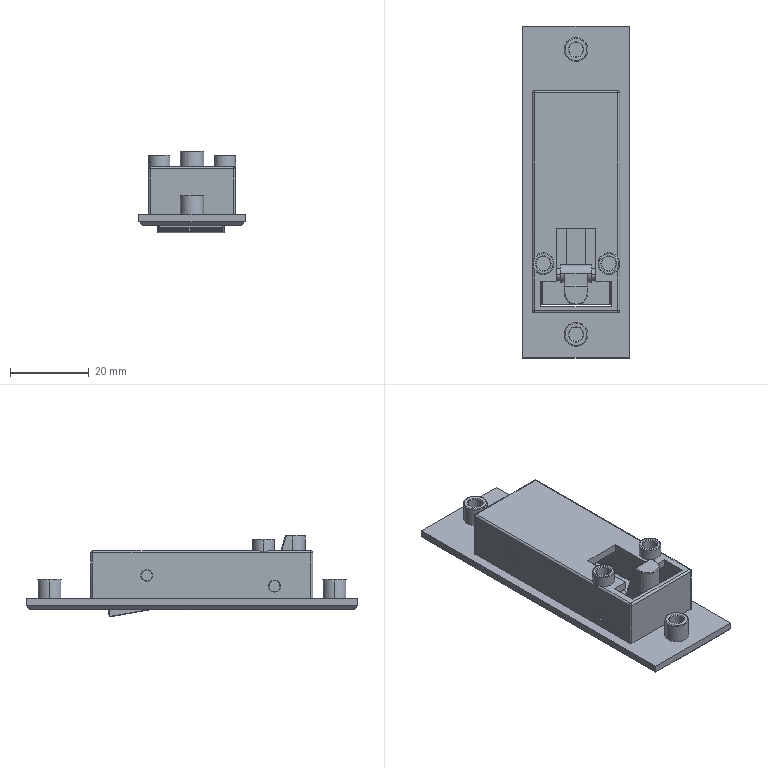Part | SolidWorks | features BaseBody 5 | 5 solids | 377 faces | box 27 x 84.5 x 20.798 mm | volume 13990 mm3 | plane 229 | cylinder 89 | spline 41 | cone 16 | torus 2 | commonest cylinder face diameters 0.4 x25 3 x16 0.2 x11 1 x11 3.6 x8 4 x5